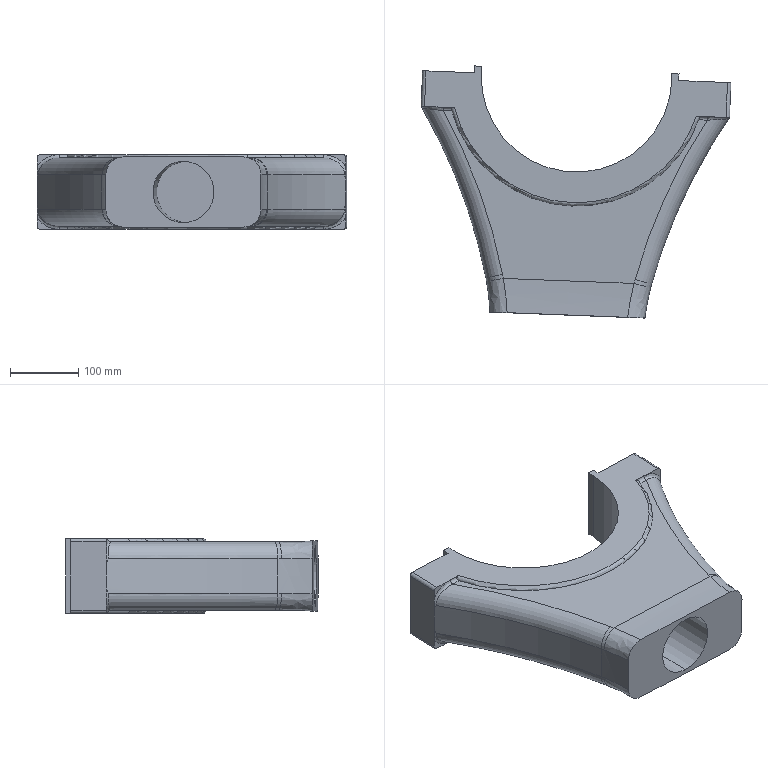Part | SolidWorks | features BaseBody 1 | 1 solid | 61 faces | box 455.294 x 369.863 x 110 mm | volume 7905953 mm3 | plane 20 | cylinder 19 | spline 16 | torus 6 | commonest cylinder face diameters 10 x8 20 x4 280 x3 90 x2 1620 x2